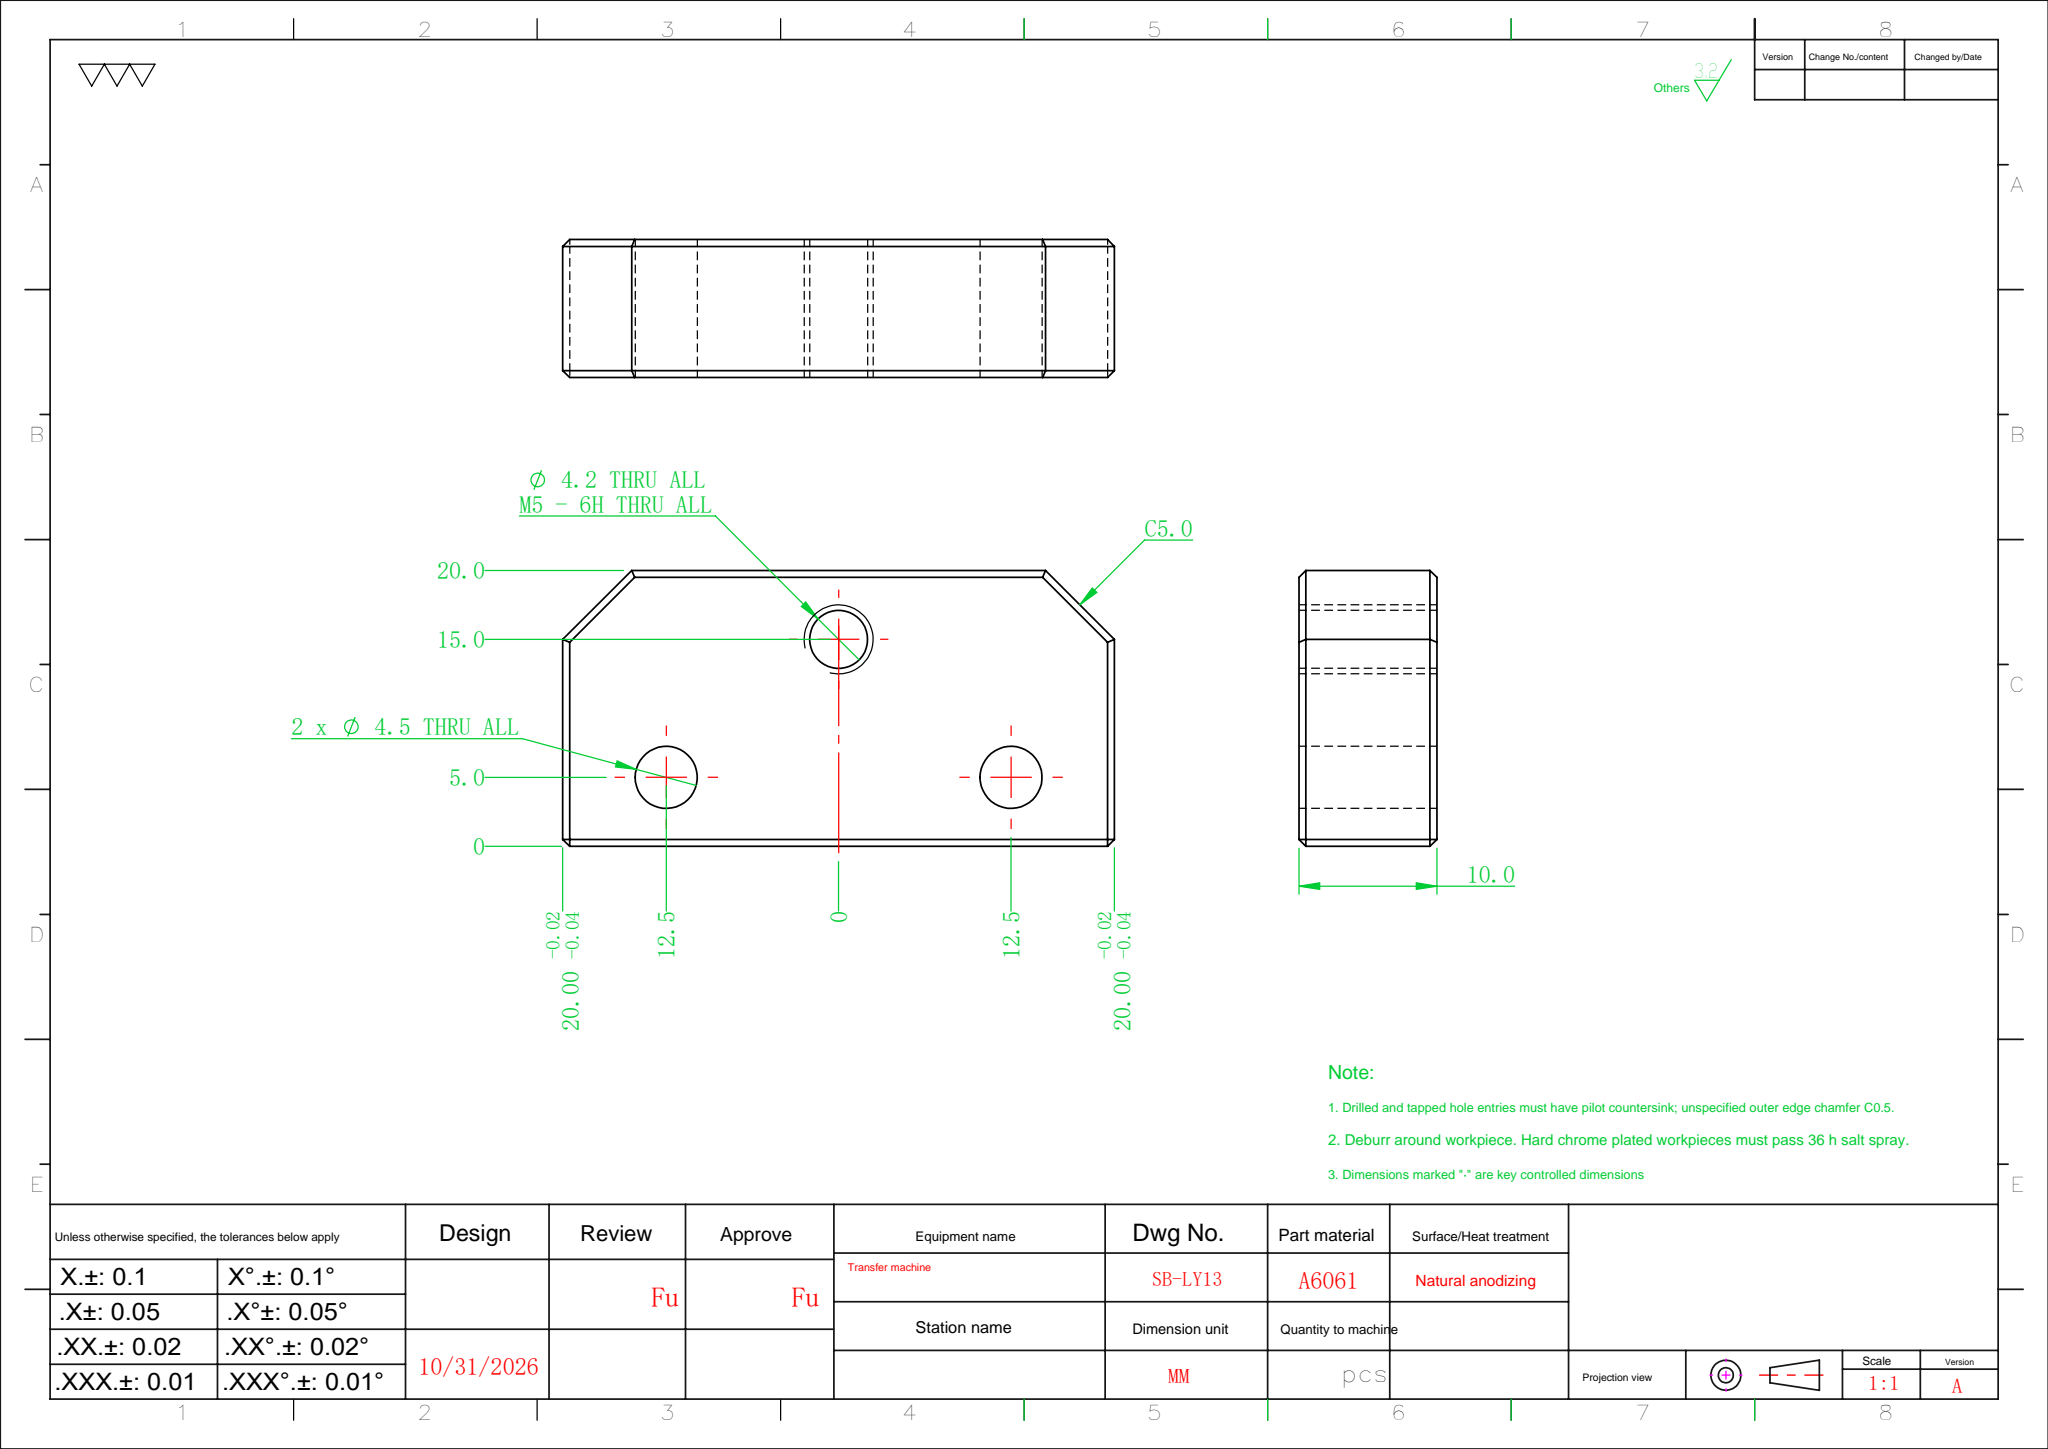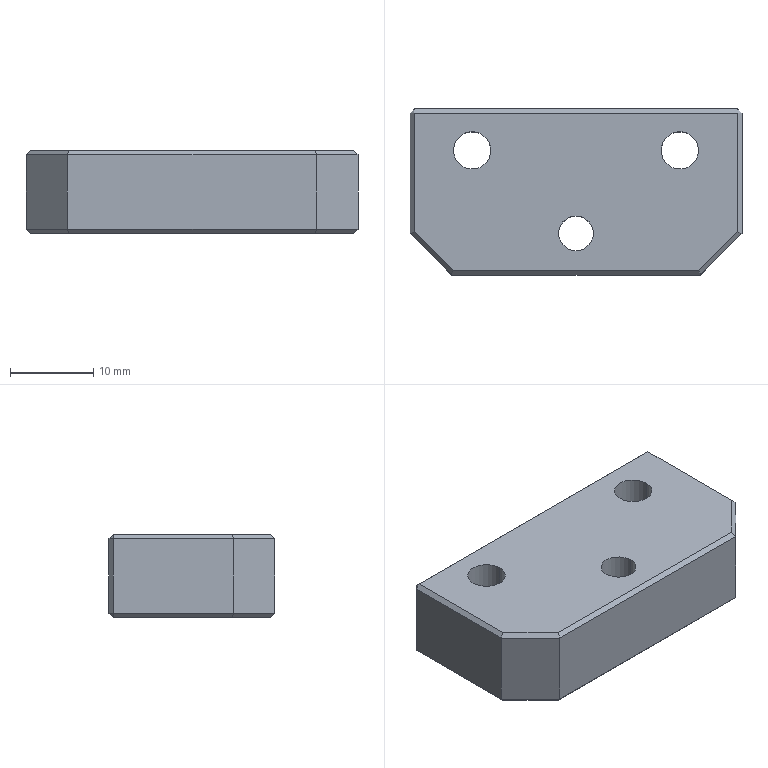Part | SolidWorks | features Chamfer 2, HoleWzd 2, Extrusion 1 | 1 solid | 32 faces | box 40 x 20 x 10 mm | volume 7263 mm3 | plane 26 | cylinder 6 | commonest cylinder face diameters 4.5 x4 4.2 x2
STEP:
#1=CARTESIAN_POINT('',(-2.1,-5.,0.));
#2=VERTEX_POINT('',#1);
#3=CARTESIAN_POINT('',(2.1,-5.,0.));
#4=VERTEX_POINT('',#3);
#5=CARTESIAN_POINT('',(0.,-5.,0.));
#6=DIRECTION('',(0.,0.,1.));
#7=DIRECTION('',(1.,0.,0.));
#8=AXIS2_PLACEMENT_3D('',#5,#6,#7);
#9=CIRCLE('',#8,2.1);
#10=EDGE_CURVE('',#2,#4,#9,.T.);
#11=ORIENTED_EDGE('',*,*,#10,.F.);
#12=CARTESIAN_POINT('',(-2.1,-5.,10.));
#13=VERTEX_POINT('',#12);
#14=CARTESIAN_POINT('',(-2.1,-5.,10.));
#15=DIRECTION('',(0.,0.,1.));
#16=VECTOR('',#15,1000.);
#17=LINE('',#14,#16);
#18=EDGE_CURVE('',#2,#13,#17,.T.);
#19=ORIENTED_EDGE('',*,*,#18,.T.);
#20=CARTESIAN_POINT('',(2.1,-5.,10.));
#21=VERTEX_POINT('',#20);
#22=CARTESIAN_POINT('',(0.,-5.,10.));
#23=DIRECTION('',(0.,0.,1.));
#24=DIRECTION('',(1.,0.,0.));
#25=AXIS2_PLACEMENT_3D('',#22,#23,#24);
#26=CIRCLE('',#25,2.1);
#27=EDGE_CURVE('',#13,#21,#26,.T.);
#28=ORIENTED_EDGE('',*,*,#27,.T.);
#29=CARTESIAN_POINT('',(2.1,-5.,10.));
#30=DIRECTION('',(0.,0.,1.));
#31=VECTOR('',#30,1000.);
#32=LINE('',#29,#31);
#33=EDGE_CURVE('',#4,#21,#32,.T.);
#34=ORIENTED_EDGE('',*,*,#33,.F.);
#35=EDGE_LOOP('',(#11,#19,#28,#34));
#36=FACE_OUTER_BOUND('',#35,.T.);
#37=CARTESIAN_POINT('',(0.,-5.,10.));
#38=DIRECTION('',(0.,0.,1.));
#39=DIRECTION('',(1.,0.,0.));
#40=AXIS2_PLACEMENT_3D('',#37,#38,#39);
#41=CYLINDRICAL_SURFACE('',#40,2.1);
#42=ADVANCED_FACE('',(#36),#41,.F.);
#43=CARTESIAN_POINT('',(10.25,5.,0.));
#44=VERTEX_POINT('',#43);
#45=CARTESIAN_POINT('',(14.75,5.,0.));
#46=VERTEX_POINT('',#45);
#47=CARTESIAN_POINT('',(12.5,5.,0.));
#48=DIRECTION('',(0.,0.,1.));
#49=DIRECTION('',(1.,0.,0.));
#50=AXIS2_PLACEMENT_3D('',#47,#48,#49);
#51=CIRCLE('',#50,2.25);
#52=EDGE_CURVE('',#44,#46,#51,.T.);
#53=ORIENTED_EDGE('',*,*,#52,.F.);
#54=CARTESIAN_POINT('',(10.25,5.,10.));
#55=VERTEX_POINT('',#54);
#56=CARTESIAN_POINT('',(10.25,5.,10.));
#57=DIRECTION('',(0.,0.,1.));
#58=VECTOR('',#57,1000.);
#59=LINE('',#56,#58);
#60=EDGE_CURVE('',#44,#55,#59,.T.);
#61=ORIENTED_EDGE('',*,*,#60,.T.);
#62=CARTESIAN_POINT('',(14.75,5.,10.));
#63=VERTEX_POINT('',#62);
#64=CARTESIAN_POINT('',(12.5,5.,10.));
#65=DIRECTION('',(0.,0.,1.));
#66=DIRECTION('',(1.,0.,0.));
#67=AXIS2_PLACEMENT_3D('',#64,#65,#66);
#68=CIRCLE('',#67,2.25);
#69=EDGE_CURVE('',#55,#63,#68,.T.);
#70=ORIENTED_EDGE('',*,*,#69,.T.);
#71=CARTESIAN_POINT('',(14.75,5.,10.));
#72=DIRECTION('',(0.,0.,1.));
#73=VECTOR('',#72,1000.);
#74=LINE('',#71,#73);
#75=EDGE_CURVE('',#46,#63,#74,.T.);
#76=ORIENTED_EDGE('',*,*,#75,.F.);
#77=EDGE_LOOP('',(#53,#61,#70,#76));
#78=FACE_OUTER_BOUND('',#77,.T.);
#79=CARTESIAN_POINT('',(12.5,5.,10.));
#80=DIRECTION('',(0.,0.,1.));
#81=DIRECTION('',(1.,0.,0.));
#82=AXIS2_PLACEMENT_3D('',#79,#80,#81);
#83=CYLINDRICAL_SURFACE('',#82,2.25);
#84=ADVANCED_FACE('',(#78),#83,.F.);
#85=CARTESIAN_POINT('',(-14.75,5.,0.));
#86=VERTEX_POINT('',#85);
#87=CARTESIAN_POINT('',(-10.25,5.,0.));
#88=VERTEX_POINT('',#87);
#89=CARTESIAN_POINT('',(-12.5,5.,0.));
#90=DIRECTION('',(0.,0.,1.));
#91=DIRECTION('',(1.,0.,0.));
#92=AXIS2_PLACEMENT_3D('',#89,#90,#91);
#93=CIRCLE('',#92,2.25);
#94=EDGE_CURVE('',#86,#88,#93,.T.);
#95=ORIENTED_EDGE('',*,*,#94,.F.);
#96=CARTESIAN_POINT('',(-14.75,5.,10.));
#97=VERTEX_POINT('',#96);
#98=CARTESIAN_POINT('',(-14.75,5.,10.));
#99=DIRECTION('',(0.,0.,1.));
#100=VECTOR('',#99,1000.);
#101=LINE('',#98,#100);
#102=EDGE_CURVE('',#86,#97,#101,.T.);
#103=ORIENTED_EDGE('',*,*,#102,.T.);
#104=CARTESIAN_POINT('',(-10.25,5.,10.));
#105=VERTEX_POINT('',#104);
#106=CARTESIAN_POINT('',(-12.5,5.,10.));
#107=DIRECTION('',(0.,0.,1.));
#108=DIRECTION('',(1.,0.,0.));
#109=AXIS2_PLACEMENT_3D('',#106,#107,#108);
#110=CIRCLE('',#109,2.25);
#111=EDGE_CURVE('',#97,#105,#110,.T.);
#112=ORIENTED_EDGE('',*,*,#111,.T.);
#113=CARTESIAN_POINT('',(-10.25,5.,10.));
#114=DIRECTION('',(0.,0.,1.));
#115=VECTOR('',#114,1000.);
#116=LINE('',#113,#115);
#117=EDGE_CURVE('',#88,#105,#116,.T.);
#118=ORIENTED_EDGE('',*,*,#117,.F.);
#119=EDGE_LOOP('',(#95,#103,#112,#118));
#120=FACE_OUTER_BOUND('',#119,.T.);
#121=CARTESIAN_POINT('',(-12.5,5.,10.));
#122=DIRECTION('',(0.,0.,1.));
#123=DIRECTION('',(1.,0.,0.));
#124=AXIS2_PLACEMENT_3D('',#121,#122,#123);
#125=CYLINDRICAL_SURFACE('',#124,2.25);
#126=ADVANCED_FACE('',(#120),#125,.F.);
#127=CARTESIAN_POINT('',(20.,-5.,9.5));
#128=VERTEX_POINT('',#127);
#129=CARTESIAN_POINT('',(20.,-5.,0.5));
#130=VERTEX_POINT('',#129);
#131=CARTESIAN_POINT('',(20.,-5.,10.));
#132=DIRECTION('',(0.,0.,-1.));
#133=VECTOR('',#132,1000.);
#134=LINE('',#131,#133);
#135=EDGE_CURVE('',#128,#130,#134,.T.);
#136=ORIENTED_EDGE('',*,*,#135,.T.);
#137=CARTESIAN_POINT('',(20.,9.5,0.5));
#138=VERTEX_POINT('',#137);
#139=CARTESIAN_POINT('',(20.,10.,0.5));
#140=DIRECTION('',(0.,1.,0.));
#141=VECTOR('',#140,1000.);
#142=LINE('',#139,#141);
#143=EDGE_CURVE('',#130,#138,#142,.T.);
#144=ORIENTED_EDGE('',*,*,#143,.T.);
#145=CARTESIAN_POINT('',(20.,9.5,9.5));
#146=VERTEX_POINT('',#145);
#147=CARTESIAN_POINT('',(20.,9.5,10.));
#148=DIRECTION('',(0.,0.,1.));
#149=VECTOR('',#148,1000.);
#150=LINE('',#147,#149);
#151=EDGE_CURVE('',#138,#146,#150,.T.);
#152=ORIENTED_EDGE('',*,*,#151,.T.);
#153=CARTESIAN_POINT('',(20.,-10.,9.5));
#154=DIRECTION('',(0.,-1.,0.));
#155=VECTOR('',#154,1000.);
#156=LINE('',#153,#155);
#157=EDGE_CURVE('',#146,#128,#156,.T.);
#158=ORIENTED_EDGE('',*,*,#157,.T.);
#159=EDGE_LOOP('',(#136,#144,#152,#158));
#160=FACE_OUTER_BOUND('',#159,.T.);
#161=CARTESIAN_POINT('',(20.,-10.,10.));
#162=DIRECTION('',(-1.,0.,0.));
#163=DIRECTION('',(0.,0.,1.));
#164=AXIS2_PLACEMENT_3D('',#161,#162,#163);
#165=PLANE('',#164);
#166=ADVANCED_FACE('',(#160),#165,.F.);
#167=CARTESIAN_POINT('',(-19.5,10.,9.5));
#168=VERTEX_POINT('',#167);
#169=CARTESIAN_POINT('',(19.5,10.,9.5));
#170=VERTEX_POINT('',#169);
#171=CARTESIAN_POINT('',(-20.,10.,9.5));
#172=DIRECTION('',(1.,0.,0.));
#173=VECTOR('',#172,1000.);
#174=LINE('',#171,#173);
#175=EDGE_CURVE('',#168,#170,#174,.T.);
#176=ORIENTED_EDGE('',*,*,#175,.T.);
#177=CARTESIAN_POINT('',(19.5,10.,0.5));
#178=VERTEX_POINT('',#177);
#179=CARTESIAN_POINT('',(19.5,10.,10.));
#180=DIRECTION('',(0.,0.,-1.));
#181=VECTOR('',#180,1000.);
#182=LINE('',#179,#181);
#183=EDGE_CURVE('',#170,#178,#182,.T.);
#184=ORIENTED_EDGE('',*,*,#183,.T.);
#185=CARTESIAN_POINT('',(-19.5,10.,0.5));
#186=VERTEX_POINT('',#185);
#187=CARTESIAN_POINT('',(-20.,10.,0.5));
#188=DIRECTION('',(-1.,0.,0.));
#189=VECTOR('',#188,1000.);
#190=LINE('',#187,#189);
#191=EDGE_CURVE('',#178,#186,#190,.T.);
#192=ORIENTED_EDGE('',*,*,#191,.T.);
#193=CARTESIAN_POINT('',(-19.5,10.,10.));
#194=DIRECTION('',(0.,0.,1.));
#195=VECTOR('',#194,1000.);
#196=LINE('',#193,#195);
#197=EDGE_CURVE('',#186,#168,#196,.T.);
#198=ORIENTED_EDGE('',*,*,#197,.T.);
#199=EDGE_LOOP('',(#176,#184,#192,#198));
#200=FACE_OUTER_BOUND('',#199,.T.);
#201=CARTESIAN_POINT('',(-20.,10.,10.));
#202=DIRECTION('',(0.,-1.,0.));
#203=DIRECTION('',(0.,0.,-1.));
#204=AXIS2_PLACEMENT_3D('',#201,#202,#203);
#205=PLANE('',#204);
#206=ADVANCED_FACE('',(#200),#205,.F.);
#207=CARTESIAN_POINT('',(-20.,9.5,9.5));
#208=VERTEX_POINT('',#207);
#209=CARTESIAN_POINT('',(-20.,9.5,0.5));
#210=VERTEX_POINT('',#209);
#211=CARTESIAN_POINT('',(-20.,9.5,10.));
#212=DIRECTION('',(0.,0.,-1.));
#213=VECTOR('',#212,1000.);
#214=LINE('',#211,#213);
#215=EDGE_CURVE('',#208,#210,#214,.T.);
#216=ORIENTED_EDGE('',*,*,#215,.T.);
#217=CARTESIAN_POINT('',(-20.,-5.,0.5));
#218=VERTEX_POINT('',#217);
#219=CARTESIAN_POINT('',(-20.,-5.,0.5));
#220=DIRECTION('',(0.,-1.,0.));
#221=VECTOR('',#220,1000.);
#222=LINE('',#219,#221);
#223=EDGE_CURVE('',#210,#218,#222,.T.);
#224=ORIENTED_EDGE('',*,*,#223,.T.);
#225=CARTESIAN_POINT('',(-20.,-5.,9.5));
#226=VERTEX_POINT('',#225);
#227=CARTESIAN_POINT('',(-20.,-5.,10.));
#228=DIRECTION('',(0.,0.,1.));
#229=VECTOR('',#228,1000.);
#230=LINE('',#227,#229);
#231=EDGE_CURVE('',#218,#226,#230,.T.);
#232=ORIENTED_EDGE('',*,*,#231,.T.);
#233=CARTESIAN_POINT('',(-20.,-10.,9.5));
#234=DIRECTION('',(0.,1.,0.));
#235=VECTOR('',#234,1000.);
#236=LINE('',#233,#235);
#237=EDGE_CURVE('',#226,#208,#236,.T.);
#238=ORIENTED_EDGE('',*,*,#237,.T.);
#239=EDGE_LOOP('',(#216,#224,#232,#238));
#240=FACE_OUTER_BOUND('',#239,.T.);
#241=CARTESIAN_POINT('',(-20.,-10.,10.));
#242=DIRECTION('',(1.,0.,0.));
#243=DIRECTION('',(0.,0.,-1.));
#244=AXIS2_PLACEMENT_3D('',#241,#242,#243);
#245=PLANE('',#244);
#246=ADVANCED_FACE('',(#240),#245,.F.);
#247=CARTESIAN_POINT('',(-15.,-10.,9.5));
#248=VERTEX_POINT('',#247);
#249=CARTESIAN_POINT('',(-15.,-10.,0.5));
#250=VERTEX_POINT('',#249);
#251=CARTESIAN_POINT('',(-15.,-10.,10.));
#252=DIRECTION('',(0.,0.,-1.));
#253=VECTOR('',#252,1000.);
#254=LINE('',#251,#253);
#255=EDGE_CURVE('',#248,#250,#254,.T.);
#256=ORIENTED_EDGE('',*,*,#255,.T.);
#257=CARTESIAN_POINT('',(15.,-10.,0.5));
#258=VERTEX_POINT('',#257);
#259=CARTESIAN_POINT('',(15.,-10.,0.5));
#260=DIRECTION('',(1.,0.,0.));
#261=VECTOR('',#260,1000.);
#262=LINE('',#259,#261);
#263=EDGE_CURVE('',#250,#258,#262,.T.);
#264=ORIENTED_EDGE('',*,*,#263,.T.);
#265=CARTESIAN_POINT('',(15.,-10.,9.5));
#266=VERTEX_POINT('',#265);
#267=CARTESIAN_POINT('',(15.,-10.,10.));
#268=DIRECTION('',(0.,0.,1.));
#269=VECTOR('',#268,1000.);
#270=LINE('',#267,#269);
#271=EDGE_CURVE('',#258,#266,#270,.T.);
#272=ORIENTED_EDGE('',*,*,#271,.T.);
#273=CARTESIAN_POINT('',(-20.,-10.,9.5));
#274=DIRECTION('',(-1.,0.,0.));
#275=VECTOR('',#274,1000.);
#276=LINE('',#273,#275);
#277=EDGE_CURVE('',#266,#248,#276,.T.);
#278=ORIENTED_EDGE('',*,*,#277,.T.);
#279=EDGE_LOOP('',(#256,#264,#272,#278));
#280=FACE_OUTER_BOUND('',#279,.T.);
#281=CARTESIAN_POINT('',(-20.,-10.,10.));
#282=DIRECTION('',(0.,1.,0.));
#283=DIRECTION('',(0.,0.,1.));
#284=AXIS2_PLACEMENT_3D('',#281,#282,#283);
#285=PLANE('',#284);
#286=ADVANCED_FACE('',(#280),#285,.F.);
#287=CARTESIAN_POINT('',(19.5,-4.793,10.));
#288=VERTEX_POINT('',#287);
#289=CARTESIAN_POINT('',(19.5,9.5,10.));
#290=VERTEX_POINT('',#289);
#291=CARTESIAN_POINT('',(19.5,0.,10.));
#292=DIRECTION('',(0.,1.,0.));
#293=VECTOR('',#292,1000.);
#294=LINE('',#291,#293);
#295=EDGE_CURVE('',#288,#290,#294,.T.);
#296=ORIENTED_EDGE('',*,*,#295,.T.);
#297=CARTESIAN_POINT('',(-19.5,9.5,10.));
#298=VERTEX_POINT('',#297);
#299=CARTESIAN_POINT('',(0.,9.5,10.));
#300=DIRECTION('',(-1.,0.,0.));
#301=VECTOR('',#300,1000.);
#302=LINE('',#299,#301);
#303=EDGE_CURVE('',#290,#298,#302,.T.);
#304=ORIENTED_EDGE('',*,*,#303,.T.);
#305=CARTESIAN_POINT('',(-19.5,-4.793,10.));
#306=VERTEX_POINT('',#305);
#307=CARTESIAN_POINT('',(-19.5,0.,10.));
#308=DIRECTION('',(0.,-1.,0.));
#309=VECTOR('',#308,1000.);
#310=LINE('',#307,#309);
#311=EDGE_CURVE('',#298,#306,#310,.T.);
#312=ORIENTED_EDGE('',*,*,#311,.T.);
#313=CARTESIAN_POINT('',(-14.793,-9.5,10.));
#314=VERTEX_POINT('',#313);
#315=CARTESIAN_POINT('',(-14.646,-9.646,10.));
#316=DIRECTION('',(0.7071,-0.7071,0.));
#317=VECTOR('',#316,1000.);
#318=LINE('',#315,#317);
#319=EDGE_CURVE('',#306,#314,#318,.T.);
#320=ORIENTED_EDGE('',*,*,#319,.T.);
#321=CARTESIAN_POINT('',(14.793,-9.5,10.));
#322=VERTEX_POINT('',#321);
#323=CARTESIAN_POINT('',(0.,-9.5,10.));
#324=DIRECTION('',(1.,0.,0.));
#325=VECTOR('',#324,1000.);
#326=LINE('',#323,#325);
#327=EDGE_CURVE('',#314,#322,#326,.T.);
#328=ORIENTED_EDGE('',*,*,#327,.T.);
#329=CARTESIAN_POINT('',(19.646,-4.646,10.));
#330=DIRECTION('',(0.7071,0.7071,0.));
#331=VECTOR('',#330,1000.);
#332=LINE('',#329,#331);
#333=EDGE_CURVE('',#322,#288,#332,.T.);
#334=ORIENTED_EDGE('',*,*,#333,.T.);
#335=EDGE_LOOP('',(#296,#304,#312,#320,#328,#334));
#336=FACE_OUTER_BOUND('',#335,.T.);
#337=CARTESIAN_POINT('',(0.,-5.,10.));
#338=DIRECTION('',(0.,0.,1.));
#339=DIRECTION('',(1.,0.,0.));
#340=AXIS2_PLACEMENT_3D('',#337,#338,#339);
#341=CIRCLE('',#340,2.1);
#342=EDGE_CURVE('',#21,#13,#341,.T.);
#343=ORIENTED_EDGE('',*,*,#342,.F.);
#344=ORIENTED_EDGE('',*,*,#27,.F.);
#345=EDGE_LOOP('',(#343,#344));
#346=FACE_BOUND('',#345,.T.);
#347=CARTESIAN_POINT('',(12.5,5.,10.));
#348=DIRECTION('',(0.,0.,1.));
#349=DIRECTION('',(1.,0.,0.));
#350=AXIS2_PLACEMENT_3D('',#347,#348,#349);
#351=CIRCLE('',#350,2.25);
#352=EDGE_CURVE('',#63,#55,#351,.T.);
#353=ORIENTED_EDGE('',*,*,#352,.F.);
#354=ORIENTED_EDGE('',*,*,#69,.F.);
#355=EDGE_LOOP('',(#353,#354));
#356=FACE_BOUND('',#355,.T.);
#357=CARTESIAN_POINT('',(-12.5,5.,10.));
#358=DIRECTION('',(0.,0.,1.));
#359=DIRECTION('',(1.,0.,0.));
#360=AXIS2_PLACEMENT_3D('',#357,#358,#359);
#361=CIRCLE('',#360,2.25);
#362=EDGE_CURVE('',#105,#97,#361,.T.);
#363=ORIENTED_EDGE('',*,*,#362,.F.);
#364=ORIENTED_EDGE('',*,*,#111,.F.);
#365=EDGE_LOOP('',(#363,#364));
#366=FACE_BOUND('',#365,.T.);
#367=CARTESIAN_POINT('',(0.,0.,10.));
#368=DIRECTION('',(0.,0.,-1.));
#369=DIRECTION('',(-1.,0.,0.));
#370=AXIS2_PLACEMENT_3D('',#367,#368,#369);
#371=PLANE('',#370);
#372=ADVANCED_FACE('',(#336,#346,#356,#366),#371,.F.);
#373=CARTESIAN_POINT('',(19.5,9.5,0.));
#374=VERTEX_POINT('',#373);
#375=CARTESIAN_POINT('',(19.5,-4.793,0.));
#376=VERTEX_POINT('',#375);
#377=CARTESIAN_POINT('',(19.5,-5.,0.));
#378=DIRECTION('',(0.,-1.,0.));
#379=VECTOR('',#378,1000.);
#380=LINE('',#377,#379);
#381=EDGE_CURVE('',#374,#376,#380,.T.);
#382=ORIENTED_EDGE('',*,*,#381,.T.);
#383=CARTESIAN_POINT('',(14.793,-9.5,0.));
#384=VERTEX_POINT('',#383);
#385=CARTESIAN_POINT('',(12.146,-12.146,0.));
#386=DIRECTION('',(-0.7071,-0.7071,0.));
#387=VECTOR('',#386,1000.);
#388=LINE('',#385,#387);
#389=EDGE_CURVE('',#376,#384,#388,.T.);
#390=ORIENTED_EDGE('',*,*,#389,.T.);
#391=CARTESIAN_POINT('',(-14.793,-9.5,0.));
#392=VERTEX_POINT('',#391);
#393=CARTESIAN_POINT('',(-15.,-9.5,0.));
#394=DIRECTION('',(-1.,0.,0.));
#395=VECTOR('',#394,1000.);
#396=LINE('',#393,#395);
#397=EDGE_CURVE('',#384,#392,#396,.T.);
#398=ORIENTED_EDGE('',*,*,#397,.T.);
#399=CARTESIAN_POINT('',(-19.5,-4.793,0.));
#400=VERTEX_POINT('',#399);
#401=CARTESIAN_POINT('',(-12.146,-12.146,0.));
#402=DIRECTION('',(-0.7071,0.7071,0.));
#403=VECTOR('',#402,1000.);
#404=LINE('',#401,#403);
#405=EDGE_CURVE('',#392,#400,#404,.T.);
#406=ORIENTED_EDGE('',*,*,#405,.T.);
#407=CARTESIAN_POINT('',(-19.5,9.5,0.));
#408=VERTEX_POINT('',#407);
#409=CARTESIAN_POINT('',(-19.5,10.,0.));
#410=DIRECTION('',(0.,1.,0.));
#411=VECTOR('',#410,1000.);
#412=LINE('',#409,#411);
#413=EDGE_CURVE('',#400,#408,#412,.T.);
#414=ORIENTED_EDGE('',*,*,#413,.T.);
#415=CARTESIAN_POINT('',(20.,9.5,0.));
#416=DIRECTION('',(1.,0.,0.));
#417=VECTOR('',#416,1000.);
#418=LINE('',#415,#417);
#419=EDGE_CURVE('',#408,#374,#418,.T.);
#420=ORIENTED_EDGE('',*,*,#419,.T.);
#421=EDGE_LOOP('',(#382,#390,#398,#406,#414,#420));
#422=FACE_OUTER_BOUND('',#421,.T.);
#423=CARTESIAN_POINT('',(0.,-5.,0.));
#424=DIRECTION('',(0.,0.,1.));
#425=DIRECTION('',(1.,0.,0.));
#426=AXIS2_PLACEMENT_3D('',#423,#424,#425);
#427=CIRCLE('',#426,2.1);
#428=EDGE_CURVE('',#4,#2,#427,.T.);
#429=ORIENTED_EDGE('',*,*,#428,.T.);
#430=ORIENTED_EDGE('',*,*,#10,.T.);
#431=EDGE_LOOP('',(#429,#430));
#432=FACE_BOUND('',#431,.T.);
#433=CARTESIAN_POINT('',(12.5,5.,0.));
#434=DIRECTION('',(0.,0.,1.));
#435=DIRECTION('',(1.,0.,0.));
#436=AXIS2_PLACEMENT_3D('',#433,#434,#435);
#437=CIRCLE('',#436,2.25);
#438=EDGE_CURVE('',#46,#44,#437,.T.);
#439=ORIENTED_EDGE('',*,*,#438,.T.);
#440=ORIENTED_EDGE('',*,*,#52,.T.);
#441=EDGE_LOOP('',(#439,#440));
#442=FACE_BOUND('',#441,.T.);
#443=CARTESIAN_POINT('',(-12.5,5.,0.));
#444=DIRECTION('',(0.,0.,1.));
#445=DIRECTION('',(1.,0.,0.));
#446=AXIS2_PLACEMENT_3D('',#443,#444,#445);
#447=CIRCLE('',#446,2.25);
#448=EDGE_CURVE('',#88,#86,#447,.T.);
#449=ORIENTED_EDGE('',*,*,#448,.T.);
#450=ORIENTED_EDGE('',*,*,#94,.T.);
#451=EDGE_LOOP('',(#449,#450));
#452=FACE_BOUND('',#451,.T.);
#453=CARTESIAN_POINT('',(0.,0.,0.));
#454=DIRECTION('',(0.,0.,-1.));
#455=DIRECTION('',(-1.,0.,0.));
#456=AXIS2_PLACEMENT_3D('',#453,#454,#455);
#457=PLANE('',#456);
#458=ADVANCED_FACE('',(#422,#432,#442,#452),#457,.T.);
#459=ORIENTED_EDGE('',*,*,#102,.F.);
#460=ORIENTED_EDGE('',*,*,#448,.F.);
#461=ORIENTED_EDGE('',*,*,#117,.T.);
#462=ORIENTED_EDGE('',*,*,#362,.T.);
#463=EDGE_LOOP('',(#459,#460,#461,#462));
#464=FACE_OUTER_BOUND('',#463,.T.);
#465=CARTESIAN_POINT('',(-12.5,5.,10.));
#466=DIRECTION('',(0.,0.,1.));
#467=DIRECTION('',(1.,0.,0.));
#468=AXIS2_PLACEMENT_3D('',#465,#466,#467);
#469=CYLINDRICAL_SURFACE('',#468,2.25);
#470=ADVANCED_FACE('',(#464),#469,.F.);
#471=ORIENTED_EDGE('',*,*,#60,.F.);
#472=ORIENTED_EDGE('',*,*,#438,.F.);
#473=ORIENTED_EDGE('',*,*,#75,.T.);
#474=ORIENTED_EDGE('',*,*,#352,.T.);
#475=EDGE_LOOP('',(#471,#472,#473,#474));
#476=FACE_OUTER_BOUND('',#475,.T.);
#477=CARTESIAN_POINT('',(12.5,5.,10.));
#478=DIRECTION('',(0.,0.,1.));
#479=DIRECTION('',(1.,0.,0.));
#480=AXIS2_PLACEMENT_3D('',#477,#478,#479);
#481=CYLINDRICAL_SURFACE('',#480,2.25);
#482=ADVANCED_FACE('',(#476),#481,.F.);
#483=ORIENTED_EDGE('',*,*,#18,.F.);
#484=ORIENTED_EDGE('',*,*,#428,.F.);
#485=ORIENTED_EDGE('',*,*,#33,.T.);
#486=ORIENTED_EDGE('',*,*,#342,.T.);
#487=EDGE_LOOP('',(#483,#484,#485,#486));
#488=FACE_OUTER_BOUND('',#487,.T.);
#489=CARTESIAN_POINT('',(0.,-5.,10.));
#490=DIRECTION('',(0.,0.,1.));
#491=DIRECTION('',(1.,0.,0.));
#492=AXIS2_PLACEMENT_3D('',#489,#490,#491);
#493=CYLINDRICAL_SURFACE('',#492,2.1);
#494=ADVANCED_FACE('',(#488),#493,.F.);
#495=ORIENTED_EDGE('',*,*,#231,.F.);
#496=CARTESIAN_POINT('',(-15.,-10.,0.5));
#497=DIRECTION('',(0.7071,-0.7071,0.));
#498=VECTOR('',#497,1000.);
#499=LINE('',#496,#498);
#500=EDGE_CURVE('',#218,#250,#499,.T.);
#501=ORIENTED_EDGE('',*,*,#500,.T.);
#502=ORIENTED_EDGE('',*,*,#255,.F.);
#503=CARTESIAN_POINT('',(-20.,-5.,9.5));
#504=DIRECTION('',(-0.7071,0.7071,0.));
#505=VECTOR('',#504,1000.);
#506=LINE('',#503,#505);
#507=EDGE_CURVE('',#248,#226,#506,.T.);
#508=ORIENTED_EDGE('',*,*,#507,.T.);
#509=EDGE_LOOP('',(#495,#501,#502,#508));
#510=FACE_OUTER_BOUND('',#509,.T.);
#511=CARTESIAN_POINT('',(-15.,-10.,10.));
#512=DIRECTION('',(0.7071,0.7071,0.));
#513=DIRECTION('',(0.,0.,-1.));
#514=AXIS2_PLACEMENT_3D('',#511,#512,#513);
#515=PLANE('',#514);
#516=ADVANCED_FACE('',(#510),#515,.F.);
#517=ORIENTED_EDGE('',*,*,#271,.F.);
#518=CARTESIAN_POINT('',(20.,-5.,0.5));
#519=DIRECTION('',(0.7071,0.7071,0.));
#520=VECTOR('',#519,1000.);
#521=LINE('',#518,#520);
#522=EDGE_CURVE('',#258,#130,#521,.T.);
#523=ORIENTED_EDGE('',*,*,#522,.T.);
#524=ORIENTED_EDGE('',*,*,#135,.F.);
#525=CARTESIAN_POINT('',(15.,-10.,9.5));
#526=DIRECTION('',(-0.7071,-0.7071,0.));
#527=VECTOR('',#526,1000.);
#528=LINE('',#525,#527);
#529=EDGE_CURVE('',#128,#266,#528,.T.);
#530=ORIENTED_EDGE('',*,*,#529,.T.);
#531=EDGE_LOOP('',(#517,#523,#524,#530));
#532=FACE_OUTER_BOUND('',#531,.T.);
#533=CARTESIAN_POINT('',(20.,-5.,10.));
#534=DIRECTION('',(-0.7071,0.7071,0.));
#535=DIRECTION('',(0.,0.,-1.));
#536=AXIS2_PLACEMENT_3D('',#533,#534,#535);
#537=PLANE('',#536);
#538=ADVANCED_FACE('',(#532),#537,.F.);
#539=CARTESIAN_POINT('',(-18.586,-4.414,10.914));
#540=DIRECTION('',(0.6786,0.2811,0.6786));
#541=VECTOR('',#540,1000.);
#542=LINE('',#539,#541);
#543=EDGE_CURVE('',#226,#306,#542,.T.);
#544=ORIENTED_EDGE('',*,*,#543,.F.);
#545=ORIENTED_EDGE('',*,*,#507,.F.);
#546=CARTESIAN_POINT('',(-15.089,-10.214,9.286));
#547=DIRECTION('',(-0.2811,-0.6786,-0.6786));
#548=VECTOR('',#547,1000.);
#549=LINE('',#546,#548);
#550=EDGE_CURVE('',#314,#248,#549,.T.);
#551=ORIENTED_EDGE('',*,*,#550,.F.);
#552=ORIENTED_EDGE('',*,*,#319,.F.);
#553=EDGE_LOOP('',(#544,#545,#551,#552));
#554=FACE_OUTER_BOUND('',#553,.T.);
#555=CARTESIAN_POINT('',(-12.146,-12.146,10.));
#556=DIRECTION('',(0.5,0.5,-0.7071));
#557=DIRECTION('',(0.7071,-0.7071,0.));
#558=AXIS2_PLACEMENT_3D('',#555,#556,#557);
#559=PLANE('',#558);
#560=ADVANCED_FACE('',(#554),#559,.F.);
#561=CARTESIAN_POINT('',(-15.089,-10.214,0.7139));
#562=DIRECTION('',(0.2811,0.6786,-0.6786));
#563=VECTOR('',#562,1000.);
#564=LINE('',#561,#563);
#565=EDGE_CURVE('',#250,#392,#564,.T.);
#566=ORIENTED_EDGE('',*,*,#565,.F.);
#567=ORIENTED_EDGE('',*,*,#500,.F.);
#568=CARTESIAN_POINT('',(-20.954,-5.395,1.454));
#569=DIRECTION('',(-0.6786,-0.2811,0.6786));
#570=VECTOR('',#569,1000.);
#571=LINE('',#568,#570);
#572=EDGE_CURVE('',#400,#218,#571,.T.);
#573=ORIENTED_EDGE('',*,*,#572,.F.);
#574=ORIENTED_EDGE('',*,*,#405,.F.);
#575=EDGE_LOOP('',(#566,#567,#573,#574));
#576=FACE_OUTER_BOUND('',#575,.T.);
#577=CARTESIAN_POINT('',(-12.146,-12.146,0.));
#578=DIRECTION('',(-0.5,-0.5,-0.7071));
#579=DIRECTION('',(0.7071,-0.7071,0.));
#580=AXIS2_PLACEMENT_3D('',#577,#578,#579);
#581=PLANE('',#580);
#582=ADVANCED_FACE('',(#576),#581,.T.);
#583=ORIENTED_EDGE('',*,*,#550,.T.);
#584=ORIENTED_EDGE('',*,*,#277,.F.);
#585=CARTESIAN_POINT('',(13.624,-6.678,12.822));
#586=DIRECTION('',(0.2811,-0.6786,-0.6786));
#587=VECTOR('',#586,1000.);
#588=LINE('',#585,#587);
#589=EDGE_CURVE('',#322,#266,#588,.T.);
#590=ORIENTED_EDGE('',*,*,#589,.F.);
#591=ORIENTED_EDGE('',*,*,#327,.F.);
#592=EDGE_LOOP('',(#583,#584,#590,#591));
#593=FACE_OUTER_BOUND('',#592,.T.);
#594=CARTESIAN_POINT('',(0.,-9.5,10.));
#595=DIRECTION('',(0.,0.7071,-0.7071));
#596=DIRECTION('',(1.,0.,0.));
#597=AXIS2_PLACEMENT_3D('',#594,#595,#596);
#598=PLANE('',#597);
#599=ADVANCED_FACE('',(#593),#598,.F.);
#600=ORIENTED_EDGE('',*,*,#543,.T.);
#601=ORIENTED_EDGE('',*,*,#311,.F.);
#602=CARTESIAN_POINT('',(-19.75,9.5,9.75));
#603=DIRECTION('',(0.7071,0.,0.7071));
#604=VECTOR('',#603,1000.);
#605=LINE('',#602,#604);
#606=EDGE_CURVE('',#208,#298,#605,.T.);
#607=ORIENTED_EDGE('',*,*,#606,.F.);
#608=ORIENTED_EDGE('',*,*,#237,.F.);
#609=EDGE_LOOP('',(#600,#601,#607,#608));
#610=FACE_OUTER_BOUND('',#609,.T.);
#611=CARTESIAN_POINT('',(-19.5,0.,10.));
#612=DIRECTION('',(0.7071,0.,-0.7071));
#613=DIRECTION('',(0.,-1.,0.));
#614=AXIS2_PLACEMENT_3D('',#611,#612,#613);
#615=PLANE('',#614);
#616=ADVANCED_FACE('',(#610),#615,.F.);
#617=CARTESIAN_POINT('',(-19.5,10.,0.5));
#618=DIRECTION('',(0.7071,0.7071,0.));
#619=VECTOR('',#618,1000.);
#620=LINE('',#617,#619);
#621=EDGE_CURVE('',#210,#186,#620,.T.);
#622=ORIENTED_EDGE('',*,*,#621,.F.);
#623=ORIENTED_EDGE('',*,*,#215,.F.);
#624=CARTESIAN_POINT('',(-19.5,10.,9.5));
#625=DIRECTION('',(-0.7071,-0.7071,0.));
#626=VECTOR('',#625,1000.);
#627=LINE('',#624,#626);
#628=EDGE_CURVE('',#168,#208,#627,.T.);
#629=ORIENTED_EDGE('',*,*,#628,.F.);
#630=ORIENTED_EDGE('',*,*,#197,.F.);
#631=EDGE_LOOP('',(#622,#623,#629,#630));
#632=FACE_OUTER_BOUND('',#631,.T.);
#633=CARTESIAN_POINT('',(-20.,9.5,10.));
#634=DIRECTION('',(0.7071,-0.7071,0.));
#635=DIRECTION('',(0.,0.,-1.));
#636=AXIS2_PLACEMENT_3D('',#633,#634,#635);
#637=PLANE('',#636);
#638=ADVANCED_FACE('',(#632),#637,.F.);
#639=ORIENTED_EDGE('',*,*,#572,.T.);
#640=ORIENTED_EDGE('',*,*,#223,.F.);
#641=CARTESIAN_POINT('',(-19.75,9.5,0.25));
#642=DIRECTION('',(-0.7071,0.,0.7071));
#643=VECTOR('',#642,1000.);
#644=LINE('',#641,#643);
#645=EDGE_CURVE('',#408,#210,#644,.T.);
#646=ORIENTED_EDGE('',*,*,#645,.F.);
#647=ORIENTED_EDGE('',*,*,#413,.F.);
#648=EDGE_LOOP('',(#639,#640,#646,#647));
#649=FACE_OUTER_BOUND('',#648,.T.);
#650=CARTESIAN_POINT('',(-20.,-10.,0.5));
#651=DIRECTION('',(-0.7071,0.,-0.7071));
#652=DIRECTION('',(0.,1.,0.));
#653=AXIS2_PLACEMENT_3D('',#650,#651,#652);
#654=PLANE('',#653);
#655=ADVANCED_FACE('',(#649),#654,.T.);
#656=ORIENTED_EDGE('',*,*,#565,.T.);
#657=ORIENTED_EDGE('',*,*,#397,.F.);
#658=CARTESIAN_POINT('',(12.235,-3.324,-6.176));
#659=DIRECTION('',(-0.2811,0.6786,-0.6786));
#660=VECTOR('',#659,1000.);
#661=LINE('',#658,#660);
#662=EDGE_CURVE('',#258,#384,#661,.T.);
#663=ORIENTED_EDGE('',*,*,#662,.F.);
#664=ORIENTED_EDGE('',*,*,#263,.F.);
#665=EDGE_LOOP('',(#656,#657,#663,#664));
#666=FACE_OUTER_BOUND('',#665,.T.);
#667=CARTESIAN_POINT('',(-20.,-10.,0.5));
#668=DIRECTION('',(0.,-0.7071,-0.7071));
#669=DIRECTION('',(-1.,0.,0.));
#670=AXIS2_PLACEMENT_3D('',#667,#668,#669);
#671=PLANE('',#670);
#672=ADVANCED_FACE('',(#666),#671,.T.);
#673=ORIENTED_EDGE('',*,*,#589,.T.);
#674=ORIENTED_EDGE('',*,*,#529,.F.);
#675=CARTESIAN_POINT('',(17.516,-3.971,11.984));
#676=DIRECTION('',(0.6786,-0.2811,-0.6786));
#677=VECTOR('',#676,1000.);
#678=LINE('',#675,#677);
#679=EDGE_CURVE('',#288,#128,#678,.T.);
#680=ORIENTED_EDGE('',*,*,#679,.F.);
#681=ORIENTED_EDGE('',*,*,#333,.F.);
#682=EDGE_LOOP('',(#673,#674,#680,#681));
#683=FACE_OUTER_BOUND('',#682,.T.);
#684=CARTESIAN_POINT('',(12.146,-12.146,10.));
#685=DIRECTION('',(-0.5,0.5,-0.7071));
#686=DIRECTION('',(0.7071,0.7071,0.));
#687=AXIS2_PLACEMENT_3D('',#684,#685,#686);
#688=PLANE('',#687);
#689=ADVANCED_FACE('',(#683),#688,.F.);
#690=ORIENTED_EDGE('',*,*,#628,.T.);
#691=ORIENTED_EDGE('',*,*,#606,.T.);
#692=CARTESIAN_POINT('',(-19.5,10.,9.5));
#693=DIRECTION('',(0.,-0.7071,0.7071));
#694=VECTOR('',#693,1000.);
#695=LINE('',#692,#694);
#696=EDGE_CURVE('',#168,#298,#695,.T.);
#697=ORIENTED_EDGE('',*,*,#696,.F.);
#698=EDGE_LOOP('',(#690,#691,#697));
#699=FACE_OUTER_BOUND('',#698,.T.);
#700=CARTESIAN_POINT('',(-19.5,10.,9.5));
#701=DIRECTION('',(-0.5774,0.5774,0.5774));
#702=DIRECTION('',(0.7071,0.,0.7071));
#703=AXIS2_PLACEMENT_3D('',#700,#701,#702);
#704=PLANE('',#703);
#705=ADVANCED_FACE('',(#699),#704,.T.);
#706=ORIENTED_EDGE('',*,*,#645,.T.);
#707=ORIENTED_EDGE('',*,*,#621,.T.);
#708=CARTESIAN_POINT('',(-19.5,10.,0.5));
#709=DIRECTION('',(0.,0.7071,0.7071));
#710=VECTOR('',#709,1000.);
#711=LINE('',#708,#710);
#712=EDGE_CURVE('',#408,#186,#711,.T.);
#713=ORIENTED_EDGE('',*,*,#712,.F.);
#714=EDGE_LOOP('',(#706,#707,#713));
#715=FACE_OUTER_BOUND('',#714,.T.);
#716=CARTESIAN_POINT('',(-19.5,10.,0.5));
#717=DIRECTION('',(-0.5774,0.5774,-0.5774));
#718=DIRECTION('',(-0.7071,0.,0.7071));
#719=AXIS2_PLACEMENT_3D('',#716,#717,#718);
#720=PLANE('',#719);
#721=ADVANCED_FACE('',(#715),#720,.T.);
#722=ORIENTED_EDGE('',*,*,#662,.T.);
#723=ORIENTED_EDGE('',*,*,#389,.F.);
#724=CARTESIAN_POINT('',(20.954,-5.395,1.454));
#725=DIRECTION('',(-0.6786,0.2811,-0.6786));
#726=VECTOR('',#725,1000.);
#727=LINE('',#724,#726);
#728=EDGE_CURVE('',#130,#376,#727,.T.);
#729=ORIENTED_EDGE('',*,*,#728,.F.);
#730=ORIENTED_EDGE('',*,*,#522,.F.);
#731=EDGE_LOOP('',(#722,#723,#729,#730));
#732=FACE_OUTER_BOUND('',#731,.T.);
#733=CARTESIAN_POINT('',(12.146,-12.146,0.));
#734=DIRECTION('',(0.5,-0.5,-0.7071));
#735=DIRECTION('',(0.7071,0.7071,0.));
#736=AXIS2_PLACEMENT_3D('',#733,#734,#735);
#737=PLANE('',#736);
#738=ADVANCED_FACE('',(#732),#737,.T.);
#739=ORIENTED_EDGE('',*,*,#679,.T.);
#740=ORIENTED_EDGE('',*,*,#157,.F.);
#741=CARTESIAN_POINT('',(20.,9.5,9.5));
#742=DIRECTION('',(0.7071,0.,-0.7071));
#743=VECTOR('',#742,1000.);
#744=LINE('',#741,#743);
#745=EDGE_CURVE('',#290,#146,#744,.T.);
#746=ORIENTED_EDGE('',*,*,#745,.F.);
#747=ORIENTED_EDGE('',*,*,#295,.F.);
#748=EDGE_LOOP('',(#739,#740,#746,#747));
#749=FACE_OUTER_BOUND('',#748,.T.);
#750=CARTESIAN_POINT('',(19.5,0.,10.));
#751=DIRECTION('',(-0.7071,0.,-0.7071));
#752=DIRECTION('',(0.,1.,0.));
#753=AXIS2_PLACEMENT_3D('',#750,#751,#752);
#754=PLANE('',#753);
#755=ADVANCED_FACE('',(#749),#754,.F.);
#756=ORIENTED_EDGE('',*,*,#696,.T.);
#757=ORIENTED_EDGE('',*,*,#303,.F.);
#758=CARTESIAN_POINT('',(19.5,9.75,9.75));
#759=DIRECTION('',(0.,-0.7071,0.7071));
#760=VECTOR('',#759,1000.);
#761=LINE('',#758,#760);
#762=EDGE_CURVE('',#170,#290,#761,.T.);
#763=ORIENTED_EDGE('',*,*,#762,.F.);
#764=ORIENTED_EDGE('',*,*,#175,.F.);
#765=EDGE_LOOP('',(#756,#757,#763,#764));
#766=FACE_OUTER_BOUND('',#765,.T.);
#767=CARTESIAN_POINT('',(0.,9.5,10.));
#768=DIRECTION('',(0.,-0.7071,-0.7071));
#769=DIRECTION('',(-1.,0.,0.));
#770=AXIS2_PLACEMENT_3D('',#767,#768,#769);
#771=PLANE('',#770);
#772=ADVANCED_FACE('',(#766),#771,.F.);
#773=ORIENTED_EDGE('',*,*,#712,.T.);
#774=ORIENTED_EDGE('',*,*,#191,.F.);
#775=CARTESIAN_POINT('',(19.5,10.,0.5));
#776=DIRECTION('',(0.,0.7071,0.7071));
#777=VECTOR('',#776,1000.);
#778=LINE('',#775,#777);
#779=EDGE_CURVE('',#374,#178,#778,.T.);
#780=ORIENTED_EDGE('',*,*,#779,.F.);
#781=ORIENTED_EDGE('',*,*,#419,.F.);
#782=EDGE_LOOP('',(#773,#774,#780,#781));
#783=FACE_OUTER_BOUND('',#782,.T.);
#784=CARTESIAN_POINT('',(-20.,10.,0.5));
#785=DIRECTION('',(0.,0.7071,-0.7071));
#786=DIRECTION('',(1.,0.,0.));
#787=AXIS2_PLACEMENT_3D('',#784,#785,#786);
#788=PLANE('',#787);
#789=ADVANCED_FACE('',(#783),#788,.T.);
#790=ORIENTED_EDGE('',*,*,#728,.T.);
#791=ORIENTED_EDGE('',*,*,#381,.F.);
#792=CARTESIAN_POINT('',(19.75,9.5,0.25));
#793=DIRECTION('',(-0.7071,0.,-0.7071));
#794=VECTOR('',#793,1000.);
#795=LINE('',#792,#794);
#796=EDGE_CURVE('',#138,#374,#795,.T.);
#797=ORIENTED_EDGE('',*,*,#796,.F.);
#798=ORIENTED_EDGE('',*,*,#143,.F.);
#799=EDGE_LOOP('',(#790,#791,#797,#798));
#800=FACE_OUTER_BOUND('',#799,.T.);
#801=CARTESIAN_POINT('',(20.,-10.,0.5));
#802=DIRECTION('',(0.7071,0.,-0.7071));
#803=DIRECTION('',(0.,-1.,0.));
#804=AXIS2_PLACEMENT_3D('',#801,#802,#803);
#805=PLANE('',#804);
#806=ADVANCED_FACE('',(#800),#805,.T.);
#807=ORIENTED_EDGE('',*,*,#762,.T.);
#808=ORIENTED_EDGE('',*,*,#745,.T.);
#809=CARTESIAN_POINT('',(20.,9.5,9.5));
#810=DIRECTION('',(0.7071,-0.7071,0.));
#811=VECTOR('',#810,1000.);
#812=LINE('',#809,#811);
#813=EDGE_CURVE('',#170,#146,#812,.T.);
#814=ORIENTED_EDGE('',*,*,#813,.F.);
#815=EDGE_LOOP('',(#807,#808,#814));
#816=FACE_OUTER_BOUND('',#815,.T.);
#817=CARTESIAN_POINT('',(20.,9.5,9.5));
#818=DIRECTION('',(0.5774,0.5774,0.5774));
#819=DIRECTION('',(0.7071,0.,-0.7071));
#820=AXIS2_PLACEMENT_3D('',#817,#818,#819);
#821=PLANE('',#820);
#822=ADVANCED_FACE('',(#816),#821,.T.);
#823=ORIENTED_EDGE('',*,*,#796,.T.);
#824=ORIENTED_EDGE('',*,*,#779,.T.);
#825=CARTESIAN_POINT('',(19.5,10.,0.5));
#826=DIRECTION('',(-0.7071,0.7071,0.));
#827=VECTOR('',#826,1000.);
#828=LINE('',#825,#827);
#829=EDGE_CURVE('',#138,#178,#828,.T.);
#830=ORIENTED_EDGE('',*,*,#829,.F.);
#831=EDGE_LOOP('',(#823,#824,#830));
#832=FACE_OUTER_BOUND('',#831,.T.);
#833=CARTESIAN_POINT('',(19.5,10.,0.5));
#834=DIRECTION('',(0.5774,0.5774,-0.5774));
#835=DIRECTION('',(-0.7071,0.,-0.7071));
#836=AXIS2_PLACEMENT_3D('',#833,#834,#835);
#837=PLANE('',#836);
#838=ADVANCED_FACE('',(#832),#837,.T.);
#839=ORIENTED_EDGE('',*,*,#813,.T.);
#840=ORIENTED_EDGE('',*,*,#151,.F.);
#841=ORIENTED_EDGE('',*,*,#829,.T.);
#842=ORIENTED_EDGE('',*,*,#183,.F.);
#843=EDGE_LOOP('',(#839,#840,#841,#842));
#844=FACE_OUTER_BOUND('',#843,.T.);
#845=CARTESIAN_POINT('',(19.5,10.,10.));
#846=DIRECTION('',(-0.7071,-0.7071,0.));
#847=DIRECTION('',(0.,0.,-1.));
#848=AXIS2_PLACEMENT_3D('',#845,#846,#847);
#849=PLANE('',#848);
#850=ADVANCED_FACE('',(#844),#849,.F.);
#851=CLOSED_SHELL('',(#42,#84,#126,#166,#206,#246,#286,#372,#458,#470,#482,#494,#516,#538,#560,#582,#599,#616,#638,#655,#672,#689,#705,#721,#738,#755,#772,#789,#806,#822,#838,#850));
#852=MANIFOLD_SOLID_BREP('',#851);
#853=CARTESIAN_POINT('',(0.,0.,0.));
#854=DIRECTION('',(0.,0.,1.));
#855=DIRECTION('',(1.,0.,0.));
#856=AXIS2_PLACEMENT_3D('',#853,#854,#855);
#857=(LENGTH_UNIT()NAMED_UNIT(*)SI_UNIT(.MILLI.,.METRE.));
#858=UNCERTAINTY_MEASURE_WITH_UNIT(LENGTH_MEASURE(0.00001),#857,'','');
#859=(NAMED_UNIT(*)PLANE_ANGLE_UNIT()SI_UNIT($,.RADIAN.));
#860=(NAMED_UNIT(*)SI_UNIT($,.STERADIAN.)SOLID_ANGLE_UNIT());
#861=(GEOMETRIC_REPRESENTATION_CONTEXT(3)GLOBAL_UNCERTAINTY_ASSIGNED_CONTEXT((#858))GLOBAL_UNIT_ASSIGNED_CONTEXT((#857,#859,#860))REPRESENTATION_CONTEXT('',''));
#862=ADVANCED_BREP_SHAPE_REPRESENTATION('',(#852,#856),#861);